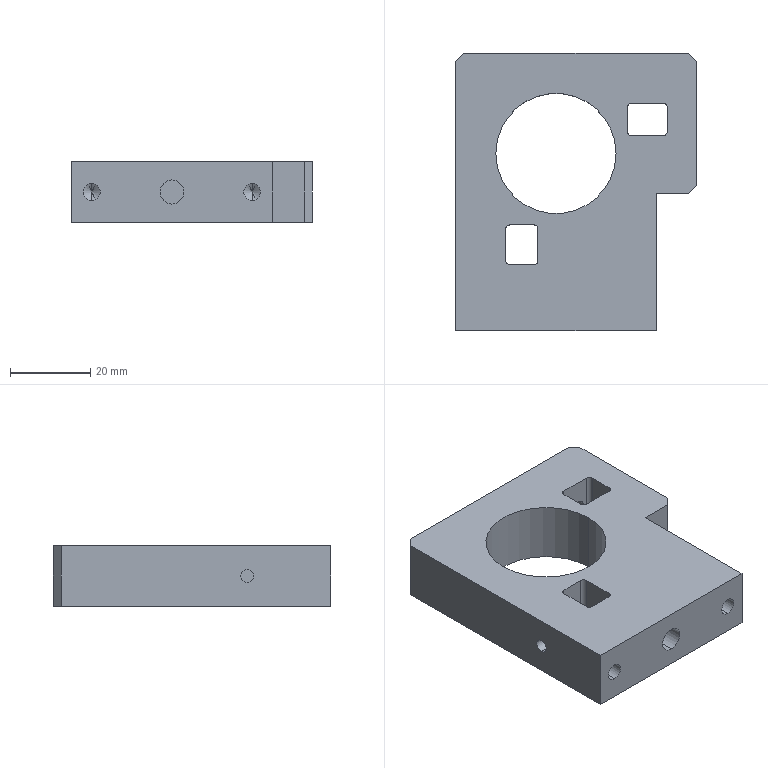Part | STEP file | 05-02-01 rotary fixing plate | 1 solid | 60 faces | box 60 x 69.2 x 15 mm | volume 42782 mm3 | cylinder 28 | plane 20 | cone 12 | commonest cylinder face diameters 3.3 x12 2 x8 4.2 x4 6 x2 30 x2